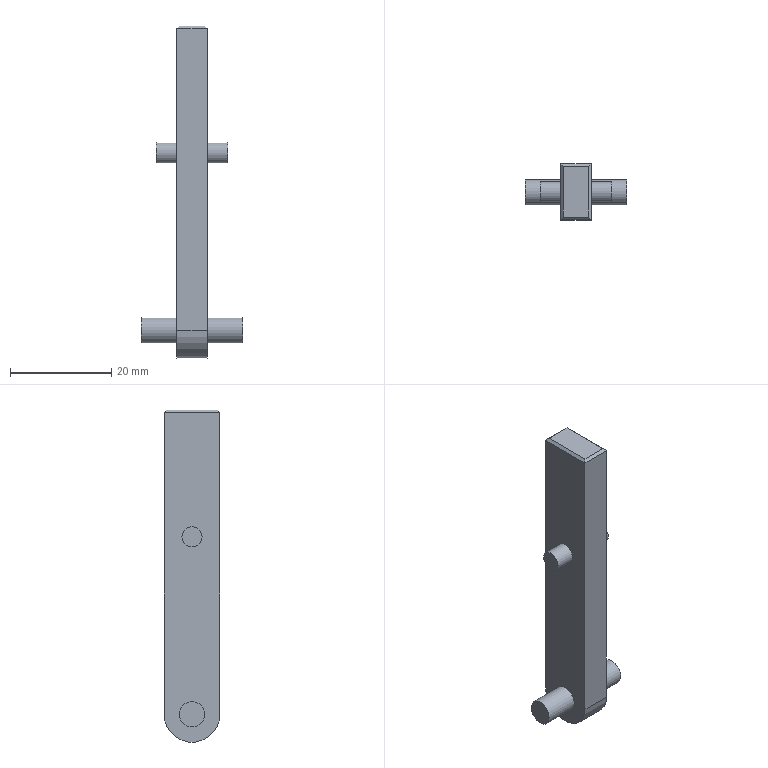Part | STEP file | 1-46.13 | 1 solid | 18 faces | box 20 x 11 x 65.5 mm | volume 4616 mm3 | plane 13 | cylinder 5 | commonest cylinder face diameters 4 x2 5 x2 11 x1
STEP:
#1=CARTESIAN_POINT('',(0.,0.,0.));
#2=DIRECTION('',(0.,0.,1.));
#3=DIRECTION('',(1.,0.,0.));
#4=AXIS2_PLACEMENT_3D('',#1,#2,#3);
#5=CARTESIAN_POINT('',(-3.,-5.5,0.));
#6=VERTEX_POINT('',#5);
#7=CARTESIAN_POINT('',(-3.,5.5,0.));
#8=VERTEX_POINT('',#7);
#9=CARTESIAN_POINT('',(-3.,0.,0.));
#10=DIRECTION('',(1.,0.,0.));
#11=DIRECTION('',(0.,-1.,0.));
#12=AXIS2_PLACEMENT_3D('',#9,#10,#11);
#13=CIRCLE('',#12,5.5);
#14=CARTESIAN_POINT('',(-3.,0.,0.));
#15=DIRECTION('',(1.,0.,0.));
#16=DIRECTION('',(0.,-1.,0.));
#17=AXIS2_PLACEMENT_3D('',#14,#15,#16);
#18=CYLINDRICAL_SURFACE('',#17,5.5);
#19=CARTESIAN_POINT('',(0.,0.));
#20=DIRECTION('',(1.,0.));
#21=VECTOR('',#20,1.);
#22=LINE('',#19,#21);
#23=(GEOMETRIC_REPRESENTATION_CONTEXT(2)PARAMETRIC_REPRESENTATION_CONTEXT()REPRESENTATION_CONTEXT('',''));
#24=DEFINITIONAL_REPRESENTATION('',(#22),#23);
#25=PCURVE('',#18,#24);
#26=CARTESIAN_POINT('',(-3.,27.25,27.25));
#27=DIRECTION('',(1.,0.,0.));
#28=DIRECTION('',(0.,1.,0.));
#29=AXIS2_PLACEMENT_3D('',#26,#27,#28);
#30=PLANE('',#29);
#31=CARTESIAN_POINT('',(-27.25,-27.25));
#32=DIRECTION('',(-1.,0.));
#33=AXIS2_PLACEMENT_2D('',#31,#32);
#34=CIRCLE('',#33,5.5);
#35=(GEOMETRIC_REPRESENTATION_CONTEXT(2)PARAMETRIC_REPRESENTATION_CONTEXT()REPRESENTATION_CONTEXT('',''));
#36=DEFINITIONAL_REPRESENTATION('',(#34),#35);
#37=PCURVE('',#30,#36);
#38=SURFACE_CURVE('',#13,(#25,#37),.PCURVE_S1.);
#39=EDGE_CURVE('',#6,#8,#38,.T.);
#40=ORIENTED_EDGE('',*,*,#39,.T.);
#41=CARTESIAN_POINT('',(3.,5.5,0.));
#42=VERTEX_POINT('',#41);
#43=CARTESIAN_POINT('',(-3.,5.5,0.));
#44=DIRECTION('',(1.,0.,0.));
#45=VECTOR('',#44,1.);
#46=LINE('',#43,#45);
#47=CARTESIAN_POINT('',(3.142,0.));
#48=DIRECTION('',(0.,1.));
#49=VECTOR('',#48,1.);
#50=LINE('',#47,#49);
#51=(GEOMETRIC_REPRESENTATION_CONTEXT(2)PARAMETRIC_REPRESENTATION_CONTEXT()REPRESENTATION_CONTEXT('',''));
#52=DEFINITIONAL_REPRESENTATION('',(#50),#51);
#53=PCURVE('',#18,#52);
#54=CARTESIAN_POINT('',(0.,5.5,30.));
#55=DIRECTION('',(0.,1.,0.));
#56=DIRECTION('',(0.,0.,1.));
#57=AXIS2_PLACEMENT_3D('',#54,#55,#56);
#58=PLANE('',#57);
#59=CARTESIAN_POINT('',(-30.,-3.));
#60=DIRECTION('',(0.,1.));
#61=VECTOR('',#60,1.);
#62=LINE('',#59,#61);
#63=(GEOMETRIC_REPRESENTATION_CONTEXT(2)PARAMETRIC_REPRESENTATION_CONTEXT()REPRESENTATION_CONTEXT('',''));
#64=DEFINITIONAL_REPRESENTATION('',(#62),#63);
#65=PCURVE('',#58,#64);
#66=SURFACE_CURVE('',#46,(#53,#65),.PCURVE_S1.);
#67=EDGE_CURVE('',#8,#42,#66,.T.);
#68=ORIENTED_EDGE('',*,*,#67,.T.);
#69=CARTESIAN_POINT('',(3.,-5.5,0.));
#70=VERTEX_POINT('',#69);
#71=CARTESIAN_POINT('',(3.,0.,0.));
#72=DIRECTION('',(1.,0.,0.));
#73=DIRECTION('',(0.,-1.,0.));
#74=AXIS2_PLACEMENT_3D('',#71,#72,#73);
#75=CIRCLE('',#74,5.5);
#76=CARTESIAN_POINT('',(0.,6.));
#77=DIRECTION('',(1.,0.));
#78=VECTOR('',#77,1.);
#79=LINE('',#76,#78);
#80=(GEOMETRIC_REPRESENTATION_CONTEXT(2)PARAMETRIC_REPRESENTATION_CONTEXT()REPRESENTATION_CONTEXT('',''));
#81=DEFINITIONAL_REPRESENTATION('',(#79),#80);
#82=PCURVE('',#18,#81);
#83=CARTESIAN_POINT('',(3.,27.25,27.25));
#84=DIRECTION('',(1.,0.,0.));
#85=DIRECTION('',(0.,1.,0.));
#86=AXIS2_PLACEMENT_3D('',#83,#84,#85);
#87=PLANE('',#86);
#88=CARTESIAN_POINT('',(-27.25,-27.25));
#89=DIRECTION('',(-1.,0.));
#90=AXIS2_PLACEMENT_2D('',#88,#89);
#91=CIRCLE('',#90,5.5);
#92=(GEOMETRIC_REPRESENTATION_CONTEXT(2)PARAMETRIC_REPRESENTATION_CONTEXT()REPRESENTATION_CONTEXT('',''));
#93=DEFINITIONAL_REPRESENTATION('',(#91),#92);
#94=PCURVE('',#87,#93);
#95=SURFACE_CURVE('',#75,(#82,#94),.PCURVE_S1.);
#96=EDGE_CURVE('',#70,#42,#95,.T.);
#97=ORIENTED_EDGE('',*,*,#96,.F.);
#98=CARTESIAN_POINT('',(-3.,-5.5,0.));
#99=DIRECTION('',(1.,0.,0.));
#100=VECTOR('',#99,1.);
#101=LINE('',#98,#100);
#102=CARTESIAN_POINT('',(0.,0.));
#103=DIRECTION('',(0.,1.));
#104=VECTOR('',#103,1.);
#105=LINE('',#102,#104);
#106=(GEOMETRIC_REPRESENTATION_CONTEXT(2)PARAMETRIC_REPRESENTATION_CONTEXT()REPRESENTATION_CONTEXT('',''));
#107=DEFINITIONAL_REPRESENTATION('',(#105),#106);
#108=PCURVE('',#18,#107);
#109=CARTESIAN_POINT('',(0.,-5.5,30.));
#110=DIRECTION('',(0.,-1.,0.));
#111=DIRECTION('',(0.,0.,-1.));
#112=AXIS2_PLACEMENT_3D('',#109,#110,#111);
#113=PLANE('',#112);
#114=CARTESIAN_POINT('',(30.,-3.));
#115=DIRECTION('',(0.,1.));
#116=VECTOR('',#115,1.);
#117=LINE('',#114,#116);
#118=(GEOMETRIC_REPRESENTATION_CONTEXT(2)PARAMETRIC_REPRESENTATION_CONTEXT()REPRESENTATION_CONTEXT('',''));
#119=DEFINITIONAL_REPRESENTATION('',(#117),#118);
#120=PCURVE('',#113,#119);
#121=SURFACE_CURVE('',#101,(#108,#120),.PCURVE_S1.);
#122=EDGE_CURVE('',#6,#70,#121,.T.);
#123=ORIENTED_EDGE('',*,*,#122,.F.);
#124=EDGE_LOOP('',(#40,#68,#97,#123));
#125=FACE_BOUND('',#124,.T.);
#126=ADVANCED_FACE('',(#125),#18,.T.);
#127=CARTESIAN_POINT('',(-7.,2.,35.));
#128=VERTEX_POINT('',#127);
#129=CARTESIAN_POINT('',(-7.,0.,35.));
#130=DIRECTION('',(1.,0.,0.));
#131=DIRECTION('',(0.,1.,0.));
#132=AXIS2_PLACEMENT_3D('',#129,#130,#131);
#133=CIRCLE('',#132,2.);
#134=CARTESIAN_POINT('',(-7.,0.,35.));
#135=DIRECTION('',(1.,0.,0.));
#136=DIRECTION('',(0.,1.,0.));
#137=AXIS2_PLACEMENT_3D('',#134,#135,#136);
#138=CYLINDRICAL_SURFACE('',#137,2.);
#139=CARTESIAN_POINT('',(0.,0.));
#140=DIRECTION('',(1.,0.));
#141=VECTOR('',#140,1.);
#142=LINE('',#139,#141);
#143=(GEOMETRIC_REPRESENTATION_CONTEXT(2)PARAMETRIC_REPRESENTATION_CONTEXT()REPRESENTATION_CONTEXT('',''));
#144=DEFINITIONAL_REPRESENTATION('',(#142),#143);
#145=PCURVE('',#138,#144);
#146=CARTESIAN_POINT('',(-7.,-0.5359,35.));
#147=DIRECTION('',(1.,0.,0.));
#148=DIRECTION('',(0.,0.,-1.));
#149=AXIS2_PLACEMENT_3D('',#146,#147,#148);
#150=PLANE('',#149);
#151=CARTESIAN_POINT('',(0.,0.5359));
#152=DIRECTION('',(0.,1.));
#153=AXIS2_PLACEMENT_2D('',#151,#152);
#154=CIRCLE('',#153,2.);
#155=(GEOMETRIC_REPRESENTATION_CONTEXT(2)PARAMETRIC_REPRESENTATION_CONTEXT()REPRESENTATION_CONTEXT('',''));
#156=DEFINITIONAL_REPRESENTATION('',(#154),#155);
#157=PCURVE('',#150,#156);
#158=SURFACE_CURVE('',#133,(#145,#157),.PCURVE_S1.);
#159=EDGE_CURVE('',#128,#128,#158,.T.);
#160=ORIENTED_EDGE('',*,*,#159,.T.);
#161=CARTESIAN_POINT('',(-3.,2.,35.));
#162=VERTEX_POINT('',#161);
#163=CARTESIAN_POINT('',(-7.,2.,35.));
#164=DIRECTION('',(1.,0.,0.));
#165=VECTOR('',#164,1.);
#166=LINE('',#163,#165);
#167=CARTESIAN_POINT('',(6.283,0.));
#168=DIRECTION('',(0.,1.));
#169=VECTOR('',#168,1.);
#170=LINE('',#167,#169);
#171=(GEOMETRIC_REPRESENTATION_CONTEXT(2)PARAMETRIC_REPRESENTATION_CONTEXT()REPRESENTATION_CONTEXT('',''));
#172=DEFINITIONAL_REPRESENTATION('',(#170),#171);
#173=PCURVE('',#138,#172);
#174=CARTESIAN_POINT('',(0.,0.));
#175=DIRECTION('',(0.,1.));
#176=VECTOR('',#175,1.);
#177=LINE('',#174,#176);
#178=(GEOMETRIC_REPRESENTATION_CONTEXT(2)PARAMETRIC_REPRESENTATION_CONTEXT()REPRESENTATION_CONTEXT('',''));
#179=DEFINITIONAL_REPRESENTATION('',(#177),#178);
#180=PCURVE('',#138,#179);
#181=SEAM_CURVE('',#166,(#173,#180),.PCURVE_S1.);
#182=EDGE_CURVE('',#128,#162,#181,.T.);
#183=ORIENTED_EDGE('',*,*,#182,.T.);
#184=CARTESIAN_POINT('',(-3.,0.,35.));
#185=DIRECTION('',(-1.,0.,0.));
#186=DIRECTION('',(0.,1.,0.));
#187=AXIS2_PLACEMENT_3D('',#184,#185,#186);
#188=CIRCLE('',#187,2.);
#189=CARTESIAN_POINT('',(6.283,4.));
#190=DIRECTION('',(-1.,0.));
#191=VECTOR('',#190,1.);
#192=LINE('',#189,#191);
#193=(GEOMETRIC_REPRESENTATION_CONTEXT(2)PARAMETRIC_REPRESENTATION_CONTEXT()REPRESENTATION_CONTEXT('',''));
#194=DEFINITIONAL_REPRESENTATION('',(#192),#193);
#195=PCURVE('',#138,#194);
#196=CARTESIAN_POINT('',(-25.25,7.75));
#197=CARTESIAN_POINT('',(-25.25,4.286));
#198=CARTESIAN_POINT('',(-28.25,6.018));
#199=CARTESIAN_POINT('',(-31.25,7.75));
#200=CARTESIAN_POINT('',(-28.25,9.482));
#201=CARTESIAN_POINT('',(-25.25,11.214));
#202=CARTESIAN_POINT('',(-25.25,7.75));
#203=(BOUNDED_CURVE()B_SPLINE_CURVE(2,(#196,#197,#198,#199,#200,#201,#202),.UNSPECIFIED.,.T.,.F.)B_SPLINE_CURVE_WITH_KNOTS((1,2,2,2,2,1),(-2.094,0.,2.094,4.189,6.283,8.378),.UNSPECIFIED.)CURVE()GEOMETRIC_REPRESENTATION_ITEM()RATIONAL_B_SPLINE_CURVE((1.,0.5,1.,0.5,1.,0.5,1.))REPRESENTATION_ITEM(''));
#204=(GEOMETRIC_REPRESENTATION_CONTEXT(2)PARAMETRIC_REPRESENTATION_CONTEXT()REPRESENTATION_CONTEXT('',''));
#205=DEFINITIONAL_REPRESENTATION('',(#203),#204);
#206=PCURVE('',#30,#205);
#207=SURFACE_CURVE('',#188,(#195,#206),.PCURVE_S1.);
#208=EDGE_CURVE('',#162,#162,#207,.T.);
#209=ORIENTED_EDGE('',*,*,#208,.T.);
#210=ORIENTED_EDGE('',*,*,#182,.F.);
#211=EDGE_LOOP('',(#160,#183,#209,#210));
#212=FACE_BOUND('',#211,.T.);
#213=ADVANCED_FACE('',(#212),#138,.T.);
#214=ORIENTED_EDGE('',*,*,#159,.T.);
#215=EDGE_LOOP('',(#214));
#216=FACE_BOUND('',#215,.F.);
#217=ADVANCED_FACE('',(#216),#150,.F.);
#218=CARTESIAN_POINT('',(7.,2.,35.));
#219=VERTEX_POINT('',#218);
#220=CARTESIAN_POINT('',(7.,0.,35.));
#221=DIRECTION('',(1.,0.,0.));
#222=DIRECTION('',(0.,1.,0.));
#223=AXIS2_PLACEMENT_3D('',#220,#221,#222);
#224=CIRCLE('',#223,2.);
#225=CARTESIAN_POINT('',(-7.,0.,35.));
#226=DIRECTION('',(1.,0.,0.));
#227=DIRECTION('',(0.,1.,0.));
#228=AXIS2_PLACEMENT_3D('',#225,#226,#227);
#229=CYLINDRICAL_SURFACE('',#228,2.);
#230=CARTESIAN_POINT('',(0.,14.));
#231=DIRECTION('',(1.,0.));
#232=VECTOR('',#231,1.);
#233=LINE('',#230,#232);
#234=(GEOMETRIC_REPRESENTATION_CONTEXT(2)PARAMETRIC_REPRESENTATION_CONTEXT()REPRESENTATION_CONTEXT('',''));
#235=DEFINITIONAL_REPRESENTATION('',(#233),#234);
#236=PCURVE('',#229,#235);
#237=CARTESIAN_POINT('',(7.,-0.5359,35.));
#238=DIRECTION('',(1.,0.,0.));
#239=DIRECTION('',(0.,0.,-1.));
#240=AXIS2_PLACEMENT_3D('',#237,#238,#239);
#241=PLANE('',#240);
#242=CARTESIAN_POINT('',(0.,0.5359));
#243=DIRECTION('',(0.,1.));
#244=AXIS2_PLACEMENT_2D('',#242,#243);
#245=CIRCLE('',#244,2.);
#246=(GEOMETRIC_REPRESENTATION_CONTEXT(2)PARAMETRIC_REPRESENTATION_CONTEXT()REPRESENTATION_CONTEXT('',''));
#247=DEFINITIONAL_REPRESENTATION('',(#245),#246);
#248=PCURVE('',#241,#247);
#249=SURFACE_CURVE('',#224,(#236,#248),.PCURVE_S1.);
#250=EDGE_CURVE('',#219,#219,#249,.T.);
#251=ORIENTED_EDGE('',*,*,#250,.F.);
#252=CARTESIAN_POINT('',(3.,2.,35.));
#253=VERTEX_POINT('',#252);
#254=CARTESIAN_POINT('',(3.,2.,35.));
#255=DIRECTION('',(1.,0.,0.));
#256=VECTOR('',#255,1.);
#257=LINE('',#254,#256);
#258=CARTESIAN_POINT('',(0.,10.));
#259=DIRECTION('',(0.,1.));
#260=VECTOR('',#259,1.);
#261=LINE('',#258,#260);
#262=(GEOMETRIC_REPRESENTATION_CONTEXT(2)PARAMETRIC_REPRESENTATION_CONTEXT()REPRESENTATION_CONTEXT('',''));
#263=DEFINITIONAL_REPRESENTATION('',(#261),#262);
#264=PCURVE('',#229,#263);
#265=CARTESIAN_POINT('',(6.283,10.));
#266=DIRECTION('',(0.,1.));
#267=VECTOR('',#266,1.);
#268=LINE('',#265,#267);
#269=(GEOMETRIC_REPRESENTATION_CONTEXT(2)PARAMETRIC_REPRESENTATION_CONTEXT()REPRESENTATION_CONTEXT('',''));
#270=DEFINITIONAL_REPRESENTATION('',(#268),#269);
#271=PCURVE('',#229,#270);
#272=SEAM_CURVE('',#257,(#264,#271),.PCURVE_S1.);
#273=EDGE_CURVE('',#253,#219,#272,.T.);
#274=ORIENTED_EDGE('',*,*,#273,.F.);
#275=CARTESIAN_POINT('',(3.,0.,35.));
#276=DIRECTION('',(-1.,0.,0.));
#277=DIRECTION('',(0.,1.,0.));
#278=AXIS2_PLACEMENT_3D('',#275,#276,#277);
#279=CIRCLE('',#278,2.);
#280=CARTESIAN_POINT('',(6.283,10.));
#281=DIRECTION('',(-1.,0.));
#282=VECTOR('',#281,1.);
#283=LINE('',#280,#282);
#284=(GEOMETRIC_REPRESENTATION_CONTEXT(2)PARAMETRIC_REPRESENTATION_CONTEXT()REPRESENTATION_CONTEXT('',''));
#285=DEFINITIONAL_REPRESENTATION('',(#283),#284);
#286=PCURVE('',#229,#285);
#287=CARTESIAN_POINT('',(-25.25,7.75));
#288=CARTESIAN_POINT('',(-25.25,4.286));
#289=CARTESIAN_POINT('',(-28.25,6.018));
#290=CARTESIAN_POINT('',(-31.25,7.75));
#291=CARTESIAN_POINT('',(-28.25,9.482));
#292=CARTESIAN_POINT('',(-25.25,11.214));
#293=CARTESIAN_POINT('',(-25.25,7.75));
#294=(BOUNDED_CURVE()B_SPLINE_CURVE(2,(#287,#288,#289,#290,#291,#292,#293),.UNSPECIFIED.,.T.,.F.)B_SPLINE_CURVE_WITH_KNOTS((1,2,2,2,2,1),(-2.094,0.,2.094,4.189,6.283,8.378),.UNSPECIFIED.)CURVE()GEOMETRIC_REPRESENTATION_ITEM()RATIONAL_B_SPLINE_CURVE((1.,0.5,1.,0.5,1.,0.5,1.))REPRESENTATION_ITEM(''));
#295=(GEOMETRIC_REPRESENTATION_CONTEXT(2)PARAMETRIC_REPRESENTATION_CONTEXT()REPRESENTATION_CONTEXT('',''));
#296=DEFINITIONAL_REPRESENTATION('',(#294),#295);
#297=PCURVE('',#87,#296);
#298=SURFACE_CURVE('',#279,(#286,#297),.PCURVE_S1.);
#299=EDGE_CURVE('',#253,#253,#298,.T.);
#300=ORIENTED_EDGE('',*,*,#299,.F.);
#301=ORIENTED_EDGE('',*,*,#273,.T.);
#302=EDGE_LOOP('',(#251,#274,#300,#301));
#303=FACE_BOUND('',#302,.T.);
#304=ADVANCED_FACE('',(#303),#229,.T.);
#305=ORIENTED_EDGE('',*,*,#250,.T.);
#306=EDGE_LOOP('',(#305));
#307=FACE_BOUND('',#306,.T.);
#308=ADVANCED_FACE('',(#307),#241,.T.);
#309=CARTESIAN_POINT('',(-10.,2.5,0.));
#310=VERTEX_POINT('',#309);
#311=CARTESIAN_POINT('',(-10.,0.,0.));
#312=DIRECTION('',(1.,0.,0.));
#313=DIRECTION('',(0.,1.,0.));
#314=AXIS2_PLACEMENT_3D('',#311,#312,#313);
#315=CIRCLE('',#314,2.5);
#316=CARTESIAN_POINT('',(-10.,0.,0.));
#317=DIRECTION('',(1.,0.,0.));
#318=DIRECTION('',(0.,1.,0.));
#319=AXIS2_PLACEMENT_3D('',#316,#317,#318);
#320=CYLINDRICAL_SURFACE('',#319,2.5);
#321=CARTESIAN_POINT('',(0.,0.));
#322=DIRECTION('',(1.,0.));
#323=VECTOR('',#322,1.);
#324=LINE('',#321,#323);
#325=(GEOMETRIC_REPRESENTATION_CONTEXT(2)PARAMETRIC_REPRESENTATION_CONTEXT()REPRESENTATION_CONTEXT('',''));
#326=DEFINITIONAL_REPRESENTATION('',(#324),#325);
#327=PCURVE('',#320,#326);
#328=CARTESIAN_POINT('',(-10.,-0.6699,0.));
#329=DIRECTION('',(1.,0.,0.));
#330=DIRECTION('',(0.,0.,-1.));
#331=AXIS2_PLACEMENT_3D('',#328,#329,#330);
#332=PLANE('',#331);
#333=CARTESIAN_POINT('',(0.,0.6699));
#334=DIRECTION('',(0.,1.));
#335=AXIS2_PLACEMENT_2D('',#333,#334);
#336=CIRCLE('',#335,2.5);
#337=(GEOMETRIC_REPRESENTATION_CONTEXT(2)PARAMETRIC_REPRESENTATION_CONTEXT()REPRESENTATION_CONTEXT('',''));
#338=DEFINITIONAL_REPRESENTATION('',(#336),#337);
#339=PCURVE('',#332,#338);
#340=SURFACE_CURVE('',#315,(#327,#339),.PCURVE_S1.);
#341=EDGE_CURVE('',#310,#310,#340,.T.);
#342=ORIENTED_EDGE('',*,*,#341,.T.);
#343=CARTESIAN_POINT('',(-3.,2.5,0.));
#344=VERTEX_POINT('',#343);
#345=CARTESIAN_POINT('',(-10.,2.5,0.));
#346=DIRECTION('',(1.,0.,0.));
#347=VECTOR('',#346,1.);
#348=LINE('',#345,#347);
#349=CARTESIAN_POINT('',(6.283,0.));
#350=DIRECTION('',(0.,1.));
#351=VECTOR('',#350,1.);
#352=LINE('',#349,#351);
#353=(GEOMETRIC_REPRESENTATION_CONTEXT(2)PARAMETRIC_REPRESENTATION_CONTEXT()REPRESENTATION_CONTEXT('',''));
#354=DEFINITIONAL_REPRESENTATION('',(#352),#353);
#355=PCURVE('',#320,#354);
#356=CARTESIAN_POINT('',(0.,0.));
#357=DIRECTION('',(0.,1.));
#358=VECTOR('',#357,1.);
#359=LINE('',#356,#358);
#360=(GEOMETRIC_REPRESENTATION_CONTEXT(2)PARAMETRIC_REPRESENTATION_CONTEXT()REPRESENTATION_CONTEXT('',''));
#361=DEFINITIONAL_REPRESENTATION('',(#359),#360);
#362=PCURVE('',#320,#361);
#363=SEAM_CURVE('',#348,(#355,#362),.PCURVE_S1.);
#364=EDGE_CURVE('',#310,#344,#363,.T.);
#365=ORIENTED_EDGE('',*,*,#364,.T.);
#366=CARTESIAN_POINT('',(-3.,0.,0.));
#367=DIRECTION('',(-1.,0.,0.));
#368=DIRECTION('',(0.,1.,0.));
#369=AXIS2_PLACEMENT_3D('',#366,#367,#368);
#370=CIRCLE('',#369,2.5);
#371=CARTESIAN_POINT('',(6.283,7.));
#372=DIRECTION('',(-1.,0.));
#373=VECTOR('',#372,1.);
#374=LINE('',#371,#373);
#375=(GEOMETRIC_REPRESENTATION_CONTEXT(2)PARAMETRIC_REPRESENTATION_CONTEXT()REPRESENTATION_CONTEXT('',''));
#376=DEFINITIONAL_REPRESENTATION('',(#374),#375);
#377=PCURVE('',#320,#376);
#378=CARTESIAN_POINT('',(-24.75,-27.25));
#379=CARTESIAN_POINT('',(-24.75,-31.58));
#380=CARTESIAN_POINT('',(-28.5,-29.415));
#381=CARTESIAN_POINT('',(-32.25,-27.25));
#382=CARTESIAN_POINT('',(-28.5,-25.085));
#383=CARTESIAN_POINT('',(-24.75,-22.92));
#384=CARTESIAN_POINT('',(-24.75,-27.25));
#385=(BOUNDED_CURVE()B_SPLINE_CURVE(2,(#378,#379,#380,#381,#382,#383,#384),.UNSPECIFIED.,.T.,.F.)B_SPLINE_CURVE_WITH_KNOTS((1,2,2,2,2,1),(-2.094,0.,2.094,4.189,6.283,8.378),.UNSPECIFIED.)CURVE()GEOMETRIC_REPRESENTATION_ITEM()RATIONAL_B_SPLINE_CURVE((1.,0.5,1.,0.5,1.,0.5,1.))REPRESENTATION_ITEM(''));
#386=(GEOMETRIC_REPRESENTATION_CONTEXT(2)PARAMETRIC_REPRESENTATION_CONTEXT()REPRESENTATION_CONTEXT('',''));
#387=DEFINITIONAL_REPRESENTATION('',(#385),#386);
#388=PCURVE('',#30,#387);
#389=SURFACE_CURVE('',#370,(#377,#388),.PCURVE_S1.);
#390=EDGE_CURVE('',#344,#344,#389,.T.);
#391=ORIENTED_EDGE('',*,*,#390,.T.);
#392=ORIENTED_EDGE('',*,*,#364,.F.);
#393=EDGE_LOOP('',(#342,#365,#391,#392));
#394=FACE_BOUND('',#393,.T.);
#395=ADVANCED_FACE('',(#394),#320,.T.);
#396=ORIENTED_EDGE('',*,*,#341,.T.);
#397=EDGE_LOOP('',(#396));
#398=FACE_BOUND('',#397,.F.);
#399=ADVANCED_FACE('',(#398),#332,.F.);
#400=CARTESIAN_POINT('',(10.,2.5,0.));
#401=VERTEX_POINT('',#400);
#402=CARTESIAN_POINT('',(10.,0.,0.));
#403=DIRECTION('',(1.,0.,0.));
#404=DIRECTION('',(0.,1.,0.));
#405=AXIS2_PLACEMENT_3D('',#402,#403,#404);
#406=CIRCLE('',#405,2.5);
#407=CARTESIAN_POINT('',(-10.,0.,0.));
#408=DIRECTION('',(1.,0.,0.));
#409=DIRECTION('',(0.,1.,0.));
#410=AXIS2_PLACEMENT_3D('',#407,#408,#409);
#411=CYLINDRICAL_SURFACE('',#410,2.5);
#412=CARTESIAN_POINT('',(0.,20.));
#413=DIRECTION('',(1.,0.));
#414=VECTOR('',#413,1.);
#415=LINE('',#412,#414);
#416=(GEOMETRIC_REPRESENTATION_CONTEXT(2)PARAMETRIC_REPRESENTATION_CONTEXT()REPRESENTATION_CONTEXT('',''));
#417=DEFINITIONAL_REPRESENTATION('',(#415),#416);
#418=PCURVE('',#411,#417);
#419=CARTESIAN_POINT('',(10.,-0.6699,0.));
#420=DIRECTION('',(1.,0.,0.));
#421=DIRECTION('',(0.,0.,-1.));
#422=AXIS2_PLACEMENT_3D('',#419,#420,#421);
#423=PLANE('',#422);
#424=CARTESIAN_POINT('',(0.,0.6699));
#425=DIRECTION('',(0.,1.));
#426=AXIS2_PLACEMENT_2D('',#424,#425);
#427=CIRCLE('',#426,2.5);
#428=(GEOMETRIC_REPRESENTATION_CONTEXT(2)PARAMETRIC_REPRESENTATION_CONTEXT()REPRESENTATION_CONTEXT('',''));
#429=DEFINITIONAL_REPRESENTATION('',(#427),#428);
#430=PCURVE('',#423,#429);
#431=SURFACE_CURVE('',#406,(#418,#430),.PCURVE_S1.);
#432=EDGE_CURVE('',#401,#401,#431,.T.);
#433=ORIENTED_EDGE('',*,*,#432,.F.);
#434=CARTESIAN_POINT('',(3.,2.5,0.));
#435=VERTEX_POINT('',#434);
#436=CARTESIAN_POINT('',(3.,2.5,0.));
#437=DIRECTION('',(1.,0.,0.));
#438=VECTOR('',#437,1.);
#439=LINE('',#436,#438);
#440=CARTESIAN_POINT('',(0.,13.));
#441=DIRECTION('',(0.,1.));
#442=VECTOR('',#441,1.);
#443=LINE('',#440,#442);
#444=(GEOMETRIC_REPRESENTATION_CONTEXT(2)PARAMETRIC_REPRESENTATION_CONTEXT()REPRESENTATION_CONTEXT('',''));
#445=DEFINITIONAL_REPRESENTATION('',(#443),#444);
#446=PCURVE('',#411,#445);
#447=CARTESIAN_POINT('',(6.283,13.));
#448=DIRECTION('',(0.,1.));
#449=VECTOR('',#448,1.);
#450=LINE('',#447,#449);
#451=(GEOMETRIC_REPRESENTATION_CONTEXT(2)PARAMETRIC_REPRESENTATION_CONTEXT()REPRESENTATION_CONTEXT('',''));
#452=DEFINITIONAL_REPRESENTATION('',(#450),#451);
#453=PCURVE('',#411,#452);
#454=SEAM_CURVE('',#439,(#446,#453),.PCURVE_S1.);
#455=EDGE_CURVE('',#435,#401,#454,.T.);
#456=ORIENTED_EDGE('',*,*,#455,.F.);
#457=CARTESIAN_POINT('',(3.,0.,0.));
#458=DIRECTION('',(-1.,0.,0.));
#459=DIRECTION('',(0.,1.,0.));
#460=AXIS2_PLACEMENT_3D('',#457,#458,#459);
#461=CIRCLE('',#460,2.5);
#462=CARTESIAN_POINT('',(6.283,13.));
#463=DIRECTION('',(-1.,0.));
#464=VECTOR('',#463,1.);
#465=LINE('',#462,#464);
#466=(GEOMETRIC_REPRESENTATION_CONTEXT(2)PARAMETRIC_REPRESENTATION_CONTEXT()REPRESENTATION_CONTEXT('',''));
#467=DEFINITIONAL_REPRESENTATION('',(#465),#466);
#468=PCURVE('',#411,#467);
#469=CARTESIAN_POINT('',(-24.75,-27.25));
#470=CARTESIAN_POINT('',(-24.75,-31.58));
#471=CARTESIAN_POINT('',(-28.5,-29.415));
#472=CARTESIAN_POINT('',(-32.25,-27.25));
#473=CARTESIAN_POINT('',(-28.5,-25.085));
#474=CARTESIAN_POINT('',(-24.75,-22.92));
#475=CARTESIAN_POINT('',(-24.75,-27.25));
#476=(BOUNDED_CURVE()B_SPLINE_CURVE(2,(#469,#470,#471,#472,#473,#474,#475),.UNSPECIFIED.,.T.,.F.)B_SPLINE_CURVE_WITH_KNOTS((1,2,2,2,2,1),(-2.094,0.,2.094,4.189,6.283,8.378),.UNSPECIFIED.)CURVE()GEOMETRIC_REPRESENTATION_ITEM()RATIONAL_B_SPLINE_CURVE((1.,0.5,1.,0.5,1.,0.5,1.))REPRESENTATION_ITEM(''));
#477=(GEOMETRIC_REPRESENTATION_CONTEXT(2)PARAMETRIC_REPRESENTATION_CONTEXT()REPRESENTATION_CONTEXT('',''));
#478=DEFINITIONAL_REPRESENTATION('',(#476),#477);
#479=PCURVE('',#87,#478);
#480=SURFACE_CURVE('',#461,(#468,#479),.PCURVE_S1.);
#481=EDGE_CURVE('',#435,#435,#480,.T.);
#482=ORIENTED_EDGE('',*,*,#481,.F.);
#483=ORIENTED_EDGE('',*,*,#455,.T.);
#484=EDGE_LOOP('',(#433,#456,#482,#483));
#485=FACE_BOUND('',#484,.T.);
#486=ADVANCED_FACE('',(#485),#411,.T.);
#487=ORIENTED_EDGE('',*,*,#432,.T.);
#488=EDGE_LOOP('',(#487));
#489=FACE_BOUND('',#488,.T.);
#490=ADVANCED_FACE('',(#489),#423,.T.);
#491=ORIENTED_EDGE('',*,*,#39,.T.);
#492=CARTESIAN_POINT('',(-3.,5.5,59.5));
#493=VERTEX_POINT('',#492);
#494=CARTESIAN_POINT('',(-3.,5.5,0.));
#495=DIRECTION('',(0.,0.,1.));
#496=VECTOR('',#495,1.);
#497=LINE('',#494,#496);
#498=CARTESIAN_POINT('',(-21.75,-27.25));
#499=DIRECTION('',(0.,1.));
#500=VECTOR('',#499,1.);
#501=LINE('',#498,#500);
#502=(GEOMETRIC_REPRESENTATION_CONTEXT(2)PARAMETRIC_REPRESENTATION_CONTEXT()REPRESENTATION_CONTEXT('',''));
#503=DEFINITIONAL_REPRESENTATION('',(#501),#502);
#504=PCURVE('',#30,#503);
#505=CARTESIAN_POINT('',(-30.,-3.));
#506=DIRECTION('',(1.,0.));
#507=VECTOR('',#506,1.);
#508=LINE('',#505,#507);
#509=(GEOMETRIC_REPRESENTATION_CONTEXT(2)PARAMETRIC_REPRESENTATION_CONTEXT()REPRESENTATION_CONTEXT('',''));
#510=DEFINITIONAL_REPRESENTATION('',(#508),#509);
#511=PCURVE('',#58,#510);
#512=SURFACE_CURVE('',#497,(#504,#511),.PCURVE_S1.);
#513=EDGE_CURVE('',#8,#493,#512,.T.);
#514=ORIENTED_EDGE('',*,*,#513,.T.);
#515=CARTESIAN_POINT('',(-3.,-5.5,59.5));
#516=VERTEX_POINT('',#515);
#517=CARTESIAN_POINT('',(-3.,5.5,59.5));
#518=DIRECTION('',(0.,-1.,0.));
#519=VECTOR('',#518,1.);
#520=LINE('',#517,#519);
#521=CARTESIAN_POINT('',(-21.75,32.25));
#522=DIRECTION('',(-1.,0.));
#523=VECTOR('',#522,1.);
#524=LINE('',#521,#523);
#525=(GEOMETRIC_REPRESENTATION_CONTEXT(2)PARAMETRIC_REPRESENTATION_CONTEXT()REPRESENTATION_CONTEXT('',''));
#526=DEFINITIONAL_REPRESENTATION('',(#524),#525);
#527=PCURVE('',#30,#526);
#528=CARTESIAN_POINT('',(-2.75,0.,59.75));
#529=DIRECTION('',(0.7071,0.,-0.7071));
#530=DIRECTION('',(0.7071,0.,0.7071));
#531=AXIS2_PLACEMENT_3D('',#528,#529,#530);
#532=PLANE('',#531);
#533=CARTESIAN_POINT('',(-0.3536,-5.5));
#534=DIRECTION('',(0.,1.));
#535=VECTOR('',#534,1.);
#536=LINE('',#533,#535);
#537=(GEOMETRIC_REPRESENTATION_CONTEXT(2)PARAMETRIC_REPRESENTATION_CONTEXT()REPRESENTATION_CONTEXT('',''));
#538=DEFINITIONAL_REPRESENTATION('',(#536),#537);
#539=PCURVE('',#532,#538);
#540=SURFACE_CURVE('',#520,(#527,#539),.PCURVE_S1.);
#541=EDGE_CURVE('',#493,#516,#540,.T.);
#542=ORIENTED_EDGE('',*,*,#541,.T.);
#543=CARTESIAN_POINT('',(-3.,-5.5,59.5));
#544=DIRECTION('',(0.,0.,-1.));
#545=VECTOR('',#544,1.);
#546=LINE('',#543,#545);
#547=CARTESIAN_POINT('',(-32.75,32.25));
#548=DIRECTION('',(0.,-1.));
#549=VECTOR('',#548,1.);
#550=LINE('',#547,#549);
#551=(GEOMETRIC_REPRESENTATION_CONTEXT(2)PARAMETRIC_REPRESENTATION_CONTEXT()REPRESENTATION_CONTEXT('',''));
#552=DEFINITIONAL_REPRESENTATION('',(#550),#551);
#553=PCURVE('',#30,#552);
#554=CARTESIAN_POINT('',(-29.5,-3.));
#555=DIRECTION('',(1.,0.));
#556=VECTOR('',#555,1.);
#557=LINE('',#554,#556);
#558=(GEOMETRIC_REPRESENTATION_CONTEXT(2)PARAMETRIC_REPRESENTATION_CONTEXT()REPRESENTATION_CONTEXT('',''));
#559=DEFINITIONAL_REPRESENTATION('',(#557),#558);
#560=PCURVE('',#113,#559);
#561=SURFACE_CURVE('',#546,(#553,#560),.PCURVE_S1.);
#562=EDGE_CURVE('',#516,#6,#561,.T.);
#563=ORIENTED_EDGE('',*,*,#562,.T.);
#564=EDGE_LOOP('',(#491,#514,#542,#563));
#565=FACE_BOUND('',#564,.F.);
#566=ORIENTED_EDGE('',*,*,#208,.T.);
#567=EDGE_LOOP('',(#566));
#568=FACE_BOUND('',#567,.F.);
#569=ORIENTED_EDGE('',*,*,#390,.T.);
#570=EDGE_LOOP('',(#569));
#571=FACE_BOUND('',#570,.F.);
#572=ADVANCED_FACE('',(#565,#568,#571),#30,.F.);
#573=ORIENTED_EDGE('',*,*,#96,.T.);
#574=CARTESIAN_POINT('',(3.,5.5,59.5));
#575=VERTEX_POINT('',#574);
#576=CARTESIAN_POINT('',(3.,5.5,0.));
#577=DIRECTION('',(0.,0.,1.));
#578=VECTOR('',#577,1.);
#579=LINE('',#576,#578);
#580=CARTESIAN_POINT('',(-21.75,-27.25));
#581=DIRECTION('',(0.,1.));
#582=VECTOR('',#581,1.);
#583=LINE('',#580,#582);
#584=(GEOMETRIC_REPRESENTATION_CONTEXT(2)PARAMETRIC_REPRESENTATION_CONTEXT()REPRESENTATION_CONTEXT('',''));
#585=DEFINITIONAL_REPRESENTATION('',(#583),#584);
#586=PCURVE('',#87,#585);
#587=CARTESIAN_POINT('',(-30.,3.));
#588=DIRECTION('',(1.,0.));
#589=VECTOR('',#588,1.);
#590=LINE('',#587,#589);
#591=(GEOMETRIC_REPRESENTATION_CONTEXT(2)PARAMETRIC_REPRESENTATION_CONTEXT()REPRESENTATION_CONTEXT('',''));
#592=DEFINITIONAL_REPRESENTATION('',(#590),#591);
#593=PCURVE('',#58,#592);
#594=SURFACE_CURVE('',#579,(#586,#593),.PCURVE_S1.);
#595=EDGE_CURVE('',#42,#575,#594,.T.);
#596=ORIENTED_EDGE('',*,*,#595,.T.);
#597=CARTESIAN_POINT('',(3.,-5.5,59.5));
#598=VERTEX_POINT('',#597);
#599=CARTESIAN_POINT('',(3.,5.5,59.5));
#600=DIRECTION('',(0.,-1.,0.));
#601=VECTOR('',#600,1.);
#602=LINE('',#599,#601);
#603=CARTESIAN_POINT('',(-21.75,32.25));
#604=DIRECTION('',(-1.,0.));
#605=VECTOR('',#604,1.);
#606=LINE('',#603,#605);
#607=(GEOMETRIC_REPRESENTATION_CONTEXT(2)PARAMETRIC_REPRESENTATION_CONTEXT()REPRESENTATION_CONTEXT('',''));
#608=DEFINITIONAL_REPRESENTATION('',(#606),#607);
#609=PCURVE('',#87,#608);
#610=CARTESIAN_POINT('',(2.75,0.,59.75));
#611=DIRECTION('',(0.7071,0.,0.7071));
#612=DIRECTION('',(-0.7071,0.,0.7071));
#613=AXIS2_PLACEMENT_3D('',#610,#611,#612);
#614=PLANE('',#613);
#615=CARTESIAN_POINT('',(-0.3536,-5.5));
#616=DIRECTION('',(0.,1.));
#617=VECTOR('',#616,1.);
#618=LINE('',#615,#617);
#619=(GEOMETRIC_REPRESENTATION_CONTEXT(2)PARAMETRIC_REPRESENTATION_CONTEXT()REPRESENTATION_CONTEXT('',''));
#620=DEFINITIONAL_REPRESENTATION('',(#618),#619);
#621=PCURVE('',#614,#620);
#622=SURFACE_CURVE('',#602,(#609,#621),.PCURVE_S1.);
#623=EDGE_CURVE('',#575,#598,#622,.T.);
#624=ORIENTED_EDGE('',*,*,#623,.T.);
#625=CARTESIAN_POINT('',(3.,-5.5,59.5));
#626=DIRECTION('',(0.,0.,-1.));
#627=VECTOR('',#626,1.);
#628=LINE('',#625,#627);
#629=CARTESIAN_POINT('',(-32.75,32.25));
#630=DIRECTION('',(0.,-1.));
#631=VECTOR('',#630,1.);
#632=LINE('',#629,#631);
#633=(GEOMETRIC_REPRESENTATION_CONTEXT(2)PARAMETRIC_REPRESENTATION_CONTEXT()REPRESENTATION_CONTEXT('',''));
#634=DEFINITIONAL_REPRESENTATION('',(#632),#633);
#635=PCURVE('',#87,#634);
#636=CARTESIAN_POINT('',(-29.5,3.));
#637=DIRECTION('',(1.,0.));
#638=VECTOR('',#637,1.);
#639=LINE('',#636,#638);
#640=(GEOMETRIC_REPRESENTATION_CONTEXT(2)PARAMETRIC_REPRESENTATION_CONTEXT()REPRESENTATION_CONTEXT('',''));
#641=DEFINITIONAL_REPRESENTATION('',(#639),#640);
#642=PCURVE('',#113,#641);
#643=SURFACE_CURVE('',#628,(#635,#642),.PCURVE_S1.);
#644=EDGE_CURVE('',#598,#70,#643,.T.);
#645=ORIENTED_EDGE('',*,*,#644,.T.);
#646=EDGE_LOOP('',(#573,#596,#624,#645));
#647=FACE_BOUND('',#646,.T.);
#648=ORIENTED_EDGE('',*,*,#299,.T.);
#649=EDGE_LOOP('',(#648));
#650=FACE_BOUND('',#649,.T.);
#651=ORIENTED_EDGE('',*,*,#481,.T.);
#652=EDGE_LOOP('',(#651));
#653=FACE_BOUND('',#652,.T.);
#654=ADVANCED_FACE('',(#647,#650,#653),#87,.T.);
#655=ORIENTED_EDGE('',*,*,#513,.T.);
#656=CARTESIAN_POINT('',(-3.,5.5,59.5));
#657=DIRECTION('',(1.,0.,0.));
#658=VECTOR('',#657,1.);
#659=LINE('',#656,#658);
#660=CARTESIAN_POINT('',(29.5,-3.));
#661=DIRECTION('',(0.,1.));
#662=VECTOR('',#661,1.);
#663=LINE('',#660,#662);
#664=(GEOMETRIC_REPRESENTATION_CONTEXT(2)PARAMETRIC_REPRESENTATION_CONTEXT()REPRESENTATION_CONTEXT('',''));
#665=DEFINITIONAL_REPRESENTATION('',(#663),#664);
#666=PCURVE('',#58,#665);
#667=CARTESIAN_POINT('',(0.,5.25,59.75));
#668=DIRECTION('',(0.,0.7071,0.7071));
#669=DIRECTION('',(0.,-0.7071,0.7071));
#670=AXIS2_PLACEMENT_3D('',#667,#668,#669);
#671=PLANE('',#670);
#672=CARTESIAN_POINT('',(-0.3536,-3.));
#673=DIRECTION('',(0.,1.));
#674=VECTOR('',#673,1.);
#675=LINE('',#672,#674);
#676=(GEOMETRIC_REPRESENTATION_CONTEXT(2)PARAMETRIC_REPRESENTATION_CONTEXT()REPRESENTATION_CONTEXT('',''));
#677=DEFINITIONAL_REPRESENTATION('',(#675),#676);
#678=PCURVE('',#671,#677);
#679=SURFACE_CURVE('',#659,(#666,#678),.PCURVE_S1.);
#680=EDGE_CURVE('',#493,#575,#679,.T.);
#681=ORIENTED_EDGE('',*,*,#680,.T.);
#682=ORIENTED_EDGE('',*,*,#595,.F.);
#683=ORIENTED_EDGE('',*,*,#67,.F.);
#684=EDGE_LOOP('',(#655,#681,#682,#683));
#685=FACE_BOUND('',#684,.T.);
#686=ADVANCED_FACE('',(#685),#58,.T.);
#687=CARTESIAN_POINT('',(-2.5,5.,60.));
#688=VERTEX_POINT('',#687);
#689=CARTESIAN_POINT('',(-2.5,-5.,60.));
#690=VERTEX_POINT('',#689);
#691=CARTESIAN_POINT('',(-2.5,5.,60.));
#692=DIRECTION('',(0.,-1.,0.));
#693=VECTOR('',#692,1.);
#694=LINE('',#691,#693);
#695=CARTESIAN_POINT('',(0.,0.,60.));
#696=DIRECTION('',(0.,0.,1.));
#697=DIRECTION('',(0.,-1.,0.));
#698=AXIS2_PLACEMENT_3D('',#695,#696,#697);
#699=PLANE('',#698);
#700=CARTESIAN_POINT('',(-5.,-2.5));
#701=DIRECTION('',(1.,0.));
#702=VECTOR('',#701,1.);
#703=LINE('',#700,#702);
#704=(GEOMETRIC_REPRESENTATION_CONTEXT(2)PARAMETRIC_REPRESENTATION_CONTEXT()REPRESENTATION_CONTEXT('',''));
#705=DEFINITIONAL_REPRESENTATION('',(#703),#704);
#706=PCURVE('',#699,#705);
#707=CARTESIAN_POINT('',(0.3536,-5.));
#708=DIRECTION('',(0.,1.));
#709=VECTOR('',#708,1.);
#710=LINE('',#707,#709);
#711=(GEOMETRIC_REPRESENTATION_CONTEXT(2)PARAMETRIC_REPRESENTATION_CONTEXT()REPRESENTATION_CONTEXT('',''));
#712=DEFINITIONAL_REPRESENTATION('',(#710),#711);
#713=PCURVE('',#532,#712);
#714=SURFACE_CURVE('',#694,(#706,#713),.PCURVE_S1.);
#715=EDGE_CURVE('',#688,#690,#714,.T.);
#716=ORIENTED_EDGE('',*,*,#715,.T.);
#717=CARTESIAN_POINT('',(2.5,-5.,60.));
#718=VERTEX_POINT('',#717);
#719=CARTESIAN_POINT('',(-2.5,-5.,60.));
#720=DIRECTION('',(1.,0.,0.));
#721=VECTOR('',#720,1.);
#722=LINE('',#719,#721);
#723=CARTESIAN_POINT('',(5.,-2.5));
#724=DIRECTION('',(0.,1.));
#725=VECTOR('',#724,1.);
#726=LINE('',#723,#725);
#727=(GEOMETRIC_REPRESENTATION_CONTEXT(2)PARAMETRIC_REPRESENTATION_CONTEXT()REPRESENTATION_CONTEXT('',''));
#728=DEFINITIONAL_REPRESENTATION('',(#726),#727);
#729=PCURVE('',#699,#728);
#730=CARTESIAN_POINT('',(0.,-5.25,59.75));
#731=DIRECTION('',(0.,-0.7071,0.7071));
#732=DIRECTION('',(0.,-0.7071,-0.7071));
#733=AXIS2_PLACEMENT_3D('',#730,#731,#732);
#734=PLANE('',#733);
#735=CARTESIAN_POINT('',(-0.3536,-2.5));
#736=DIRECTION('',(0.,1.));
#737=VECTOR('',#736,1.);
#738=LINE('',#735,#737);
#739=(GEOMETRIC_REPRESENTATION_CONTEXT(2)PARAMETRIC_REPRESENTATION_CONTEXT()REPRESENTATION_CONTEXT('',''));
#740=DEFINITIONAL_REPRESENTATION('',(#738),#739);
#741=PCURVE('',#734,#740);
#742=SURFACE_CURVE('',#722,(#729,#741),.PCURVE_S1.);
#743=EDGE_CURVE('',#690,#718,#742,.T.);
#744=ORIENTED_EDGE('',*,*,#743,.T.);
#745=CARTESIAN_POINT('',(2.5,5.,60.));
#746=VERTEX_POINT('',#745);
#747=CARTESIAN_POINT('',(2.5,5.,60.));
#748=DIRECTION('',(0.,-1.,0.));
#749=VECTOR('',#748,1.);
#750=LINE('',#747,#749);
#751=CARTESIAN_POINT('',(-5.,2.5));
#752=DIRECTION('',(1.,0.));
#753=VECTOR('',#752,1.);
#754=LINE('',#751,#753);
#755=(GEOMETRIC_REPRESENTATION_CONTEXT(2)PARAMETRIC_REPRESENTATION_CONTEXT()REPRESENTATION_CONTEXT('',''));
#756=DEFINITIONAL_REPRESENTATION('',(#754),#755);
#757=PCURVE('',#699,#756);
#758=CARTESIAN_POINT('',(0.3536,-5.));
#759=DIRECTION('',(0.,1.));
#760=VECTOR('',#759,1.);
#761=LINE('',#758,#760);
#762=(GEOMETRIC_REPRESENTATION_CONTEXT(2)PARAMETRIC_REPRESENTATION_CONTEXT()REPRESENTATION_CONTEXT('',''));
#763=DEFINITIONAL_REPRESENTATION('',(#761),#762);
#764=PCURVE('',#614,#763);
#765=SURFACE_CURVE('',#750,(#757,#764),.PCURVE_S1.);
#766=EDGE_CURVE('',#746,#718,#765,.T.);
#767=ORIENTED_EDGE('',*,*,#766,.F.);
#768=CARTESIAN_POINT('',(-2.5,5.,60.));
#769=DIRECTION('',(1.,0.,0.));
#770=VECTOR('',#769,1.);
#771=LINE('',#768,#770);
#772=CARTESIAN_POINT('',(-5.,-2.5));
#773=DIRECTION('',(0.,1.));
#774=VECTOR('',#773,1.);
#775=LINE('',#772,#774);
#776=(GEOMETRIC_REPRESENTATION_CONTEXT(2)PARAMETRIC_REPRESENTATION_CONTEXT()REPRESENTATION_CONTEXT('',''));
#777=DEFINITIONAL_REPRESENTATION('',(#775),#776);
#778=PCURVE('',#699,#777);
#779=CARTESIAN_POINT('',(0.3536,-2.5));
#780=DIRECTION('',(0.,1.));
#781=VECTOR('',#780,1.);
#782=LINE('',#779,#781);
#783=(GEOMETRIC_REPRESENTATION_CONTEXT(2)PARAMETRIC_REPRESENTATION_CONTEXT()REPRESENTATION_CONTEXT('',''));
#784=DEFINITIONAL_REPRESENTATION('',(#782),#783);
#785=PCURVE('',#671,#784);
#786=SURFACE_CURVE('',#771,(#778,#785),.PCURVE_S1.);
#787=EDGE_CURVE('',#688,#746,#786,.T.);
#788=ORIENTED_EDGE('',*,*,#787,.F.);
#789=EDGE_LOOP('',(#716,#744,#767,#788));
#790=FACE_BOUND('',#789,.T.);
#791=ADVANCED_FACE('',(#790),#699,.T.);
#792=ORIENTED_EDGE('',*,*,#644,.F.);
#793=CARTESIAN_POINT('',(-3.,-5.5,59.5));
#794=DIRECTION('',(1.,0.,0.));
#795=VECTOR('',#794,1.);
#796=LINE('',#793,#795);
#797=CARTESIAN_POINT('',(-29.5,-3.));
#798=DIRECTION('',(0.,1.));
#799=VECTOR('',#798,1.);
#800=LINE('',#797,#799);
#801=(GEOMETRIC_REPRESENTATION_CONTEXT(2)PARAMETRIC_REPRESENTATION_CONTEXT()REPRESENTATION_CONTEXT('',''));
#802=DEFINITIONAL_REPRESENTATION('',(#800),#801);
#803=PCURVE('',#113,#802);
#804=CARTESIAN_POINT('',(0.3536,-3.));
#805=DIRECTION('',(0.,1.));
#806=VECTOR('',#805,1.);
#807=LINE('',#804,#806);
#808=(GEOMETRIC_REPRESENTATION_CONTEXT(2)PARAMETRIC_REPRESENTATION_CONTEXT()REPRESENTATION_CONTEXT('',''));
#809=DEFINITIONAL_REPRESENTATION('',(#807),#808);
#810=PCURVE('',#734,#809);
#811=SURFACE_CURVE('',#796,(#803,#810),.PCURVE_S1.);
#812=EDGE_CURVE('',#516,#598,#811,.T.);
#813=ORIENTED_EDGE('',*,*,#812,.F.);
#814=ORIENTED_EDGE('',*,*,#562,.T.);
#815=ORIENTED_EDGE('',*,*,#122,.T.);
#816=EDGE_LOOP('',(#792,#813,#814,#815));
#817=FACE_BOUND('',#816,.T.);
#818=ADVANCED_FACE('',(#817),#113,.T.);
#819=ORIENTED_EDGE('',*,*,#541,.F.);
#820=CARTESIAN_POINT('',(-3.,5.5,59.5));
#821=DIRECTION('',(0.5774,-0.5774,0.5774));
#822=VECTOR('',#821,1.);
#823=LINE('',#820,#822);
#824=CARTESIAN_POINT('',(-0.3536,-5.5));
#825=DIRECTION('',(0.8165,0.5774));
#826=VECTOR('',#825,1.);
#827=LINE('',#824,#826);
#828=(GEOMETRIC_REPRESENTATION_CONTEXT(2)PARAMETRIC_REPRESENTATION_CONTEXT()REPRESENTATION_CONTEXT('',''));
#829=DEFINITIONAL_REPRESENTATION('',(#827),#828);
#830=PCURVE('',#532,#829);
#831=CARTESIAN_POINT('',(-0.3536,-3.));
#832=DIRECTION('',(0.8165,0.5774));
#833=VECTOR('',#832,1.);
#834=LINE('',#831,#833);
#835=(GEOMETRIC_REPRESENTATION_CONTEXT(2)PARAMETRIC_REPRESENTATION_CONTEXT()REPRESENTATION_CONTEXT('',''));
#836=DEFINITIONAL_REPRESENTATION('',(#834),#835);
#837=PCURVE('',#671,#836);
#838=SURFACE_CURVE('',#823,(#830,#837),.PCURVE_S1.);
#839=EDGE_CURVE('',#493,#688,#838,.T.);
#840=ORIENTED_EDGE('',*,*,#839,.T.);
#841=ORIENTED_EDGE('',*,*,#715,.T.);
#842=CARTESIAN_POINT('',(-3.,-5.5,59.5));
#843=DIRECTION('',(0.5774,0.5774,0.5774));
#844=VECTOR('',#843,1.);
#845=LINE('',#842,#844);
#846=CARTESIAN_POINT('',(-0.3536,5.5));
#847=DIRECTION('',(0.8165,-0.5774));
#848=VECTOR('',#847,1.);
#849=LINE('',#846,#848);
#850=(GEOMETRIC_REPRESENTATION_CONTEXT(2)PARAMETRIC_REPRESENTATION_CONTEXT()REPRESENTATION_CONTEXT('',''));
#851=DEFINITIONAL_REPRESENTATION('',(#849),#850);
#852=PCURVE('',#532,#851);
#853=CARTESIAN_POINT('',(0.3536,-3.));
#854=DIRECTION('',(-0.8165,0.5774));
#855=VECTOR('',#854,1.);
#856=LINE('',#853,#855);
#857=(GEOMETRIC_REPRESENTATION_CONTEXT(2)PARAMETRIC_REPRESENTATION_CONTEXT()REPRESENTATION_CONTEXT('',''));
#858=DEFINITIONAL_REPRESENTATION('',(#856),#857);
#859=PCURVE('',#734,#858);
#860=SURFACE_CURVE('',#845,(#852,#859),.PCURVE_S1.);
#861=EDGE_CURVE('',#516,#690,#860,.T.);
#862=ORIENTED_EDGE('',*,*,#861,.F.);
#863=EDGE_LOOP('',(#819,#840,#841,#862));
#864=FACE_BOUND('',#863,.F.);
#865=ADVANCED_FACE('',(#864),#532,.F.);
#866=ORIENTED_EDGE('',*,*,#623,.F.);
#867=CARTESIAN_POINT('',(3.,5.5,59.5));
#868=DIRECTION('',(-0.5774,-0.5774,0.5774));
#869=VECTOR('',#868,1.);
#870=LINE('',#867,#869);
#871=CARTESIAN_POINT('',(-0.3536,-5.5));
#872=DIRECTION('',(0.8165,0.5774));
#873=VECTOR('',#872,1.);
#874=LINE('',#871,#873);
#875=(GEOMETRIC_REPRESENTATION_CONTEXT(2)PARAMETRIC_REPRESENTATION_CONTEXT()REPRESENTATION_CONTEXT('',''));
#876=DEFINITIONAL_REPRESENTATION('',(#874),#875);
#877=PCURVE('',#614,#876);
#878=CARTESIAN_POINT('',(-0.3536,3.));
#879=DIRECTION('',(0.8165,-0.5774));
#880=VECTOR('',#879,1.);
#881=LINE('',#878,#880);
#882=(GEOMETRIC_REPRESENTATION_CONTEXT(2)PARAMETRIC_REPRESENTATION_CONTEXT()REPRESENTATION_CONTEXT('',''));
#883=DEFINITIONAL_REPRESENTATION('',(#881),#882);
#884=PCURVE('',#671,#883);
#885=SURFACE_CURVE('',#870,(#877,#884),.PCURVE_S1.);
#886=EDGE_CURVE('',#575,#746,#885,.T.);
#887=ORIENTED_EDGE('',*,*,#886,.T.);
#888=ORIENTED_EDGE('',*,*,#766,.T.);
#889=CARTESIAN_POINT('',(3.,-5.5,59.5));
#890=DIRECTION('',(-0.5774,0.5774,0.5774));
#891=VECTOR('',#890,1.);
#892=LINE('',#889,#891);
#893=CARTESIAN_POINT('',(-0.3536,5.5));
#894=DIRECTION('',(0.8165,-0.5774));
#895=VECTOR('',#894,1.);
#896=LINE('',#893,#895);
#897=(GEOMETRIC_REPRESENTATION_CONTEXT(2)PARAMETRIC_REPRESENTATION_CONTEXT()REPRESENTATION_CONTEXT('',''));
#898=DEFINITIONAL_REPRESENTATION('',(#896),#897);
#899=PCURVE('',#614,#898);
#900=CARTESIAN_POINT('',(0.3536,3.));
#901=DIRECTION('',(-0.8165,-0.5774));
#902=VECTOR('',#901,1.);
#903=LINE('',#900,#902);
#904=(GEOMETRIC_REPRESENTATION_CONTEXT(2)PARAMETRIC_REPRESENTATION_CONTEXT()REPRESENTATION_CONTEXT('',''));
#905=DEFINITIONAL_REPRESENTATION('',(#903),#904);
#906=PCURVE('',#734,#905);
#907=SURFACE_CURVE('',#892,(#899,#906),.PCURVE_S1.);
#908=EDGE_CURVE('',#598,#718,#907,.T.);
#909=ORIENTED_EDGE('',*,*,#908,.F.);
#910=EDGE_LOOP('',(#866,#887,#888,#909));
#911=FACE_BOUND('',#910,.T.);
#912=ADVANCED_FACE('',(#911),#614,.T.);
#913=ORIENTED_EDGE('',*,*,#680,.F.);
#914=ORIENTED_EDGE('',*,*,#839,.T.);
#915=ORIENTED_EDGE('',*,*,#787,.T.);
#916=ORIENTED_EDGE('',*,*,#886,.F.);
#917=EDGE_LOOP('',(#913,#914,#915,#916));
#918=FACE_BOUND('',#917,.T.);
#919=ADVANCED_FACE('',(#918),#671,.T.);
#920=ORIENTED_EDGE('',*,*,#812,.T.);
#921=ORIENTED_EDGE('',*,*,#908,.T.);
#922=ORIENTED_EDGE('',*,*,#743,.F.);
#923=ORIENTED_EDGE('',*,*,#861,.F.);
#924=EDGE_LOOP('',(#920,#921,#922,#923));
#925=FACE_BOUND('',#924,.T.);
#926=ADVANCED_FACE('',(#925),#734,.T.);
#927=CLOSED_SHELL('',(#126,#213,#217,#304,#308,#395,#399,#486,#490,#572,#654,#686,#791,#818,#865,#912,#919,#926));
#928=MANIFOLD_SOLID_BREP('',#927);
#929=(LENGTH_UNIT()NAMED_UNIT(*)SI_UNIT(.MILLI.,.METRE.));
#930=UNCERTAINTY_MEASURE_WITH_UNIT(LENGTH_MEASURE(0.0000001),#929,'','');
#931=(NAMED_UNIT(*)PLANE_ANGLE_UNIT()SI_UNIT($,.RADIAN.));
#932=(NAMED_UNIT(*)SI_UNIT($,.STERADIAN.)SOLID_ANGLE_UNIT());
#933=(GEOMETRIC_REPRESENTATION_CONTEXT(3)GLOBAL_UNCERTAINTY_ASSIGNED_CONTEXT((#930))GLOBAL_UNIT_ASSIGNED_CONTEXT((#929,#931,#932))REPRESENTATION_CONTEXT('',''));
#934=ADVANCED_BREP_SHAPE_REPRESENTATION('',(#4,#928),#933);